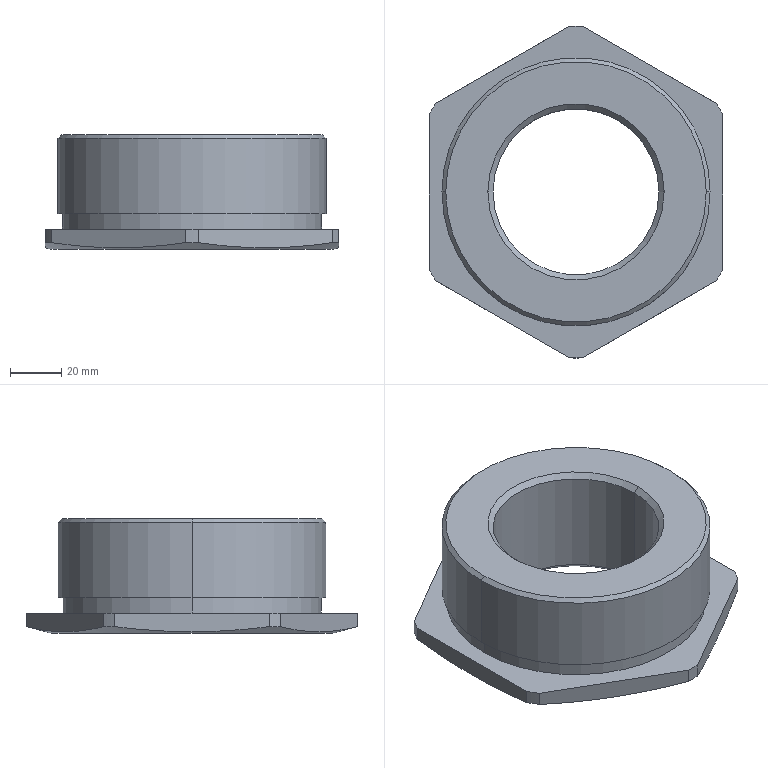Part | SolidWorks | features ICE 4, Chamfer 2, Extrusion 1 | 1 solid | 30 faces | box 115 x 130 x 45 mm | volume 256191 mm3 | cylinder 12 | plane 10 | cone 8 | commonest cylinder face diameters 130 x6 65 x2 101.5 x2 105 x2
STEP:
#1=CARTESIAN_POINT('',(55.,0.,0.));
#2=VERTEX_POINT('',#1);
#3=CARTESIAN_POINT('',(-55.,0.,0.));
#4=VERTEX_POINT('',#3);
#5=CARTESIAN_POINT('',(0.,0.,0.));
#6=DIRECTION('',(0.,0.,-1.));
#7=DIRECTION('',(-1.,0.,0.));
#8=AXIS2_PLACEMENT_3D('',#5,#6,#7);
#9=CIRCLE('',#8,55.);
#10=EDGE_CURVE('',#2,#4,#9,.T.);
#11=ORIENTED_EDGE('',*,*,#10,.F.);
#12=CARTESIAN_POINT('',(57.5,0.,0.6699));
#13=VERTEX_POINT('',#12);
#14=CARTESIAN_POINT('',(55.,0.,0.));
#15=DIRECTION('',(0.9659,0.,0.2588));
#16=VECTOR('',#15,1000.);
#17=LINE('',#14,#16);
#18=EDGE_CURVE('',#2,#13,#17,.T.);
#19=ORIENTED_EDGE('',*,*,#18,.T.);
#20=CARTESIAN_POINT('',(57.5,-30.311,2.679));
#21=VERTEX_POINT('',#20);
#22=CARTESIAN_POINT('',(57.5,0.,0.6699));
#23=CARTESIAN_POINT('',(57.5,-5.026,0.6699));
#24=CARTESIAN_POINT('',(57.5,-10.072,0.8493));
#25=CARTESIAN_POINT('',(57.5,-17.671,1.368));
#26=CARTESIAN_POINT('',(57.5,-20.211,1.582));
#27=CARTESIAN_POINT('',(57.5,-25.27,2.08));
#28=CARTESIAN_POINT('',(57.5,-27.793,2.365));
#29=CARTESIAN_POINT('',(57.5,-30.311,2.679));
#30=B_SPLINE_CURVE_WITH_KNOTS('',3,(#22,#23,#24,#25,#26,#27,#28,#29),.UNSPECIFIED.,.F.,.F.,(4,2,2,4),(0.09241,0.1074,0.1149,0.1224),.UNSPECIFIED.);
#31=EDGE_CURVE('',#13,#21,#30,.T.);
#32=ORIENTED_EDGE('',*,*,#31,.T.);
#33=CARTESIAN_POINT('',(55.,-34.641,2.679));
#34=VERTEX_POINT('',#33);
#35=CARTESIAN_POINT('',(0.,0.,2.679));
#36=DIRECTION('',(0.,0.,-1.));
#37=DIRECTION('',(1.,0.,0.));
#38=AXIS2_PLACEMENT_3D('',#35,#36,#37);
#39=CIRCLE('',#38,65.);
#40=EDGE_CURVE('',#21,#34,#39,.T.);
#41=ORIENTED_EDGE('',*,*,#40,.T.);
#42=CARTESIAN_POINT('',(2.5,-64.952,2.679));
#43=VERTEX_POINT('',#42);
#44=CARTESIAN_POINT('',(55.,-34.641,2.679));
#45=CARTESIAN_POINT('',(50.625,-37.167,2.048));
#46=CARTESIAN_POINT('',(46.25,-39.693,1.541));
#47=CARTESIAN_POINT('',(37.5,-44.745,0.8511));
#48=CARTESIAN_POINT('',(28.75,-49.796,0.4887));
#49=CARTESIAN_POINT('',(20.,-54.848,0.8511));
#50=CARTESIAN_POINT('',(11.25,-59.9,1.541));
#51=CARTESIAN_POINT('',(6.875,-62.426,2.048));
#52=CARTESIAN_POINT('',(2.5,-64.952,2.679));
#53=B_SPLINE_CURVE_WITH_KNOTS('',3,(#44,#45,#46,#47,#48,#49,#50,#51,#52),.UNSPECIFIED.,.F.,.F.,(4,2,1,2,4),(0.000000231,0.01516,0.03031,0.04547,0.06062),.UNSPECIFIED.);
#54=EDGE_CURVE('',#34,#43,#53,.T.);
#55=ORIENTED_EDGE('',*,*,#54,.T.);
#56=CARTESIAN_POINT('',(-2.5,-64.952,2.679));
#57=VERTEX_POINT('',#56);
#58=CARTESIAN_POINT('',(0.,0.,2.679));
#59=DIRECTION('',(0.,0.,-1.));
#60=DIRECTION('',(1.,0.,0.));
#61=AXIS2_PLACEMENT_3D('',#58,#59,#60);
#62=CIRCLE('',#61,65.);
#63=EDGE_CURVE('',#43,#57,#62,.T.);
#64=ORIENTED_EDGE('',*,*,#63,.T.);
#65=CARTESIAN_POINT('',(-55.,-34.641,2.679));
#66=VERTEX_POINT('',#65);
#67=CARTESIAN_POINT('',(-2.5,-64.952,2.679));
#68=CARTESIAN_POINT('',(-6.875,-62.426,2.048));
#69=CARTESIAN_POINT('',(-11.25,-59.9,1.541));
#70=CARTESIAN_POINT('',(-20.,-54.848,0.8511));
#71=CARTESIAN_POINT('',(-28.75,-49.796,0.4887));
#72=CARTESIAN_POINT('',(-37.5,-44.745,0.8511));
#73=CARTESIAN_POINT('',(-46.25,-39.693,1.541));
#74=CARTESIAN_POINT('',(-50.625,-37.167,2.048));
#75=CARTESIAN_POINT('',(-55.,-34.641,2.679));
#76=B_SPLINE_CURVE_WITH_KNOTS('',3,(#67,#68,#69,#70,#71,#72,#73,#74,#75),.UNSPECIFIED.,.F.,.F.,(4,2,1,2,4),(0.000000231,0.01516,0.03031,0.04547,0.06062),.UNSPECIFIED.);
#77=EDGE_CURVE('',#57,#66,#76,.T.);
#78=ORIENTED_EDGE('',*,*,#77,.T.);
#79=CARTESIAN_POINT('',(-57.5,-30.311,2.679));
#80=VERTEX_POINT('',#79);
#81=CARTESIAN_POINT('',(0.,0.,2.679));
#82=DIRECTION('',(0.,0.,-1.));
#83=DIRECTION('',(1.,0.,0.));
#84=AXIS2_PLACEMENT_3D('',#81,#82,#83);
#85=CIRCLE('',#84,65.);
#86=EDGE_CURVE('',#66,#80,#85,.T.);
#87=ORIENTED_EDGE('',*,*,#86,.T.);
#88=CARTESIAN_POINT('',(-57.5,0.,0.6699));
#89=VERTEX_POINT('',#88);
#90=CARTESIAN_POINT('',(-57.5,-30.311,2.679));
#91=CARTESIAN_POINT('',(-57.5,-25.293,2.053));
#92=CARTESIAN_POINT('',(-57.5,-20.261,1.546));
#93=CARTESIAN_POINT('',(-57.5,-10.16,0.8538));
#94=CARTESIAN_POINT('',(-57.5,-5.091,0.6699));
#95=CARTESIAN_POINT('',(-57.5,0.,0.6699));
#96=B_SPLINE_CURVE_WITH_KNOTS('',3,(#90,#91,#92,#93,#94,#95),.UNSPECIFIED.,.F.,.F.,(4,2,4),(0.06207,0.07724,0.09241),.UNSPECIFIED.);
#97=EDGE_CURVE('',#80,#89,#96,.T.);
#98=ORIENTED_EDGE('',*,*,#97,.T.);
#99=CARTESIAN_POINT('',(-55.,0.,0.));
#100=DIRECTION('',(-0.9659,0.,0.2588));
#101=VECTOR('',#100,1000.);
#102=LINE('',#99,#101);
#103=EDGE_CURVE('',#4,#89,#102,.T.);
#104=ORIENTED_EDGE('',*,*,#103,.F.);
#105=EDGE_LOOP('',(#11,#19,#32,#41,#55,#64,#78,#87,#98,#104));
#106=FACE_OUTER_BOUND('',#105,.T.);
#107=CARTESIAN_POINT('',(0.,0.,0.));
#108=DIRECTION('',(0.,0.,1.));
#109=DIRECTION('',(-1.,0.,0.));
#110=AXIS2_PLACEMENT_3D('',#107,#108,#109);
#111=CONICAL_SURFACE('',#110,55.,1.309);
#112=ADVANCED_FACE('',(#106),#111,.T.);
#113=CARTESIAN_POINT('',(51.,0.,45.));
#114=VERTEX_POINT('',#113);
#115=CARTESIAN_POINT('',(-51.,0.,45.));
#116=VERTEX_POINT('',#115);
#117=CARTESIAN_POINT('',(0.,0.,45.));
#118=DIRECTION('',(0.,0.,1.));
#119=DIRECTION('',(-1.,0.,0.));
#120=AXIS2_PLACEMENT_3D('',#117,#118,#119);
#121=CIRCLE('',#120,51.);
#122=EDGE_CURVE('',#114,#116,#121,.T.);
#123=ORIENTED_EDGE('',*,*,#122,.F.);
#124=CARTESIAN_POINT('',(52.5,0.,43.5));
#125=VERTEX_POINT('',#124);
#126=CARTESIAN_POINT('',(52.5,0.,43.5));
#127=DIRECTION('',(0.7071,0.,-0.7071));
#128=VECTOR('',#127,1000.);
#129=LINE('',#126,#128);
#130=EDGE_CURVE('',#114,#125,#129,.T.);
#131=ORIENTED_EDGE('',*,*,#130,.T.);
#132=CARTESIAN_POINT('',(-52.5,0.,43.5));
#133=VERTEX_POINT('',#132);
#134=CARTESIAN_POINT('',(0.,0.,43.5));
#135=DIRECTION('',(0.,0.,-1.));
#136=DIRECTION('',(-1.,0.,0.));
#137=AXIS2_PLACEMENT_3D('',#134,#135,#136);
#138=CIRCLE('',#137,52.5);
#139=EDGE_CURVE('',#133,#125,#138,.T.);
#140=ORIENTED_EDGE('',*,*,#139,.F.);
#141=CARTESIAN_POINT('',(-52.5,0.,43.5));
#142=DIRECTION('',(-0.7071,0.,-0.7071));
#143=VECTOR('',#142,1000.);
#144=LINE('',#141,#143);
#145=EDGE_CURVE('',#116,#133,#144,.T.);
#146=ORIENTED_EDGE('',*,*,#145,.F.);
#147=EDGE_LOOP('',(#123,#131,#140,#146));
#148=FACE_OUTER_BOUND('',#147,.T.);
#149=CARTESIAN_POINT('',(0.,0.,43.5));
#150=DIRECTION('',(0.,0.,-1.));
#151=DIRECTION('',(-1.,0.,0.));
#152=AXIS2_PLACEMENT_3D('',#149,#150,#151);
#153=CONICAL_SURFACE('',#152,52.5,0.7854);
#154=ADVANCED_FACE('',(#148),#153,.T.);
#155=CARTESIAN_POINT('',(32.5,0.,2.));
#156=VERTEX_POINT('',#155);
#157=CARTESIAN_POINT('',(-32.5,0.,2.));
#158=VERTEX_POINT('',#157);
#159=CARTESIAN_POINT('',(0.,0.,2.));
#160=DIRECTION('',(0.,0.,-1.));
#161=DIRECTION('',(1.,0.,0.));
#162=AXIS2_PLACEMENT_3D('',#159,#160,#161);
#163=CIRCLE('',#162,32.5);
#164=EDGE_CURVE('',#156,#158,#163,.T.);
#165=ORIENTED_EDGE('',*,*,#164,.F.);
#166=CARTESIAN_POINT('',(34.5,0.,0.));
#167=VERTEX_POINT('',#166);
#168=CARTESIAN_POINT('',(34.5,0.,0.));
#169=DIRECTION('',(0.7071,0.,-0.7071));
#170=VECTOR('',#169,1000.);
#171=LINE('',#168,#170);
#172=EDGE_CURVE('',#156,#167,#171,.T.);
#173=ORIENTED_EDGE('',*,*,#172,.T.);
#174=CARTESIAN_POINT('',(-34.5,0.,0.));
#175=VERTEX_POINT('',#174);
#176=CARTESIAN_POINT('',(0.,0.,0.));
#177=DIRECTION('',(0.,0.,1.));
#178=DIRECTION('',(1.,0.,0.));
#179=AXIS2_PLACEMENT_3D('',#176,#177,#178);
#180=CIRCLE('',#179,34.5);
#181=EDGE_CURVE('',#175,#167,#180,.T.);
#182=ORIENTED_EDGE('',*,*,#181,.F.);
#183=CARTESIAN_POINT('',(-34.5,0.,0.));
#184=DIRECTION('',(-0.7071,0.,-0.7071));
#185=VECTOR('',#184,1000.);
#186=LINE('',#183,#185);
#187=EDGE_CURVE('',#158,#175,#186,.T.);
#188=ORIENTED_EDGE('',*,*,#187,.F.);
#189=EDGE_LOOP('',(#165,#173,#182,#188));
#190=FACE_OUTER_BOUND('',#189,.T.);
#191=CARTESIAN_POINT('',(0.,0.,0.));
#192=DIRECTION('',(0.,0.,-1.));
#193=DIRECTION('',(-1.,0.,0.));
#194=AXIS2_PLACEMENT_3D('',#191,#192,#193);
#195=CONICAL_SURFACE('',#194,34.5,0.7854);
#196=ADVANCED_FACE('',(#190),#195,.F.);
#197=CARTESIAN_POINT('',(-32.5,0.,43.));
#198=VERTEX_POINT('',#197);
#199=CARTESIAN_POINT('',(32.5,0.,43.));
#200=VERTEX_POINT('',#199);
#201=CARTESIAN_POINT('',(0.,0.,43.));
#202=DIRECTION('',(0.,0.,1.));
#203=DIRECTION('',(-1.,0.,0.));
#204=AXIS2_PLACEMENT_3D('',#201,#202,#203);
#205=CIRCLE('',#204,32.5);
#206=EDGE_CURVE('',#198,#200,#205,.T.);
#207=ORIENTED_EDGE('',*,*,#206,.F.);
#208=CARTESIAN_POINT('',(-34.5,0.,45.));
#209=VERTEX_POINT('',#208);
#210=CARTESIAN_POINT('',(-32.5,0.,43.));
#211=DIRECTION('',(-0.7071,0.,0.7071));
#212=VECTOR('',#211,1000.);
#213=LINE('',#210,#212);
#214=EDGE_CURVE('',#198,#209,#213,.T.);
#215=ORIENTED_EDGE('',*,*,#214,.T.);
#216=CARTESIAN_POINT('',(34.5,0.,45.));
#217=VERTEX_POINT('',#216);
#218=CARTESIAN_POINT('',(0.,0.,45.));
#219=DIRECTION('',(0.,0.,-1.));
#220=DIRECTION('',(-1.,0.,0.));
#221=AXIS2_PLACEMENT_3D('',#218,#219,#220);
#222=CIRCLE('',#221,34.5);
#223=EDGE_CURVE('',#217,#209,#222,.T.);
#224=ORIENTED_EDGE('',*,*,#223,.F.);
#225=CARTESIAN_POINT('',(32.5,0.,43.));
#226=DIRECTION('',(0.7071,0.,0.7071));
#227=VECTOR('',#226,1000.);
#228=LINE('',#225,#227);
#229=EDGE_CURVE('',#200,#217,#228,.T.);
#230=ORIENTED_EDGE('',*,*,#229,.F.);
#231=EDGE_LOOP('',(#207,#215,#224,#230));
#232=FACE_OUTER_BOUND('',#231,.T.);
#233=CARTESIAN_POINT('',(0.,0.,43.));
#234=DIRECTION('',(0.,0.,1.));
#235=DIRECTION('',(1.,0.,0.));
#236=AXIS2_PLACEMENT_3D('',#233,#234,#235);
#237=CONICAL_SURFACE('',#236,32.5,0.7854);
#238=ADVANCED_FACE('',(#232),#237,.F.);
#239=ORIENTED_EDGE('',*,*,#164,.T.);
#240=CARTESIAN_POINT('',(-32.5,0.,0.));
#241=DIRECTION('',(0.,0.,1.));
#242=VECTOR('',#241,1000.);
#243=LINE('',#240,#242);
#244=EDGE_CURVE('',#158,#198,#243,.T.);
#245=ORIENTED_EDGE('',*,*,#244,.T.);
#246=ORIENTED_EDGE('',*,*,#206,.T.);
#247=CARTESIAN_POINT('',(32.5,0.,0.));
#248=DIRECTION('',(0.,0.,1.));
#249=VECTOR('',#248,1000.);
#250=LINE('',#247,#249);
#251=EDGE_CURVE('',#156,#200,#250,.T.);
#252=ORIENTED_EDGE('',*,*,#251,.F.);
#253=EDGE_LOOP('',(#239,#245,#246,#252));
#254=FACE_OUTER_BOUND('',#253,.T.);
#255=CARTESIAN_POINT('',(0.,0.,0.));
#256=DIRECTION('',(0.,0.,1.));
#257=DIRECTION('',(1.,0.,0.));
#258=AXIS2_PLACEMENT_3D('',#255,#256,#257);
#259=CYLINDRICAL_SURFACE('',#258,32.5);
#260=ADVANCED_FACE('',(#254),#259,.F.);
#261=ORIENTED_EDGE('',*,*,#139,.T.);
#262=CARTESIAN_POINT('',(52.5,0.,14.));
#263=VERTEX_POINT('',#262);
#264=CARTESIAN_POINT('',(52.5,0.,45.));
#265=DIRECTION('',(0.,0.,-1.));
#266=VECTOR('',#265,1000.);
#267=LINE('',#264,#266);
#268=EDGE_CURVE('',#125,#263,#267,.T.);
#269=ORIENTED_EDGE('',*,*,#268,.T.);
#270=CARTESIAN_POINT('',(-52.5,0.,14.));
#271=VERTEX_POINT('',#270);
#272=CARTESIAN_POINT('',(0.,0.,14.));
#273=DIRECTION('',(0.,0.,1.));
#274=DIRECTION('',(1.,0.,0.));
#275=AXIS2_PLACEMENT_3D('',#272,#273,#274);
#276=CIRCLE('',#275,52.5);
#277=EDGE_CURVE('',#263,#271,#276,.T.);
#278=ORIENTED_EDGE('',*,*,#277,.T.);
#279=CARTESIAN_POINT('',(-52.5,0.,45.));
#280=DIRECTION('',(0.,0.,-1.));
#281=VECTOR('',#280,1000.);
#282=LINE('',#279,#281);
#283=EDGE_CURVE('',#133,#271,#282,.T.);
#284=ORIENTED_EDGE('',*,*,#283,.F.);
#285=EDGE_LOOP('',(#261,#269,#278,#284));
#286=FACE_OUTER_BOUND('',#285,.T.);
#287=CARTESIAN_POINT('',(0.,0.,45.));
#288=DIRECTION('',(0.,0.,-1.));
#289=DIRECTION('',(-1.,0.,0.));
#290=AXIS2_PLACEMENT_3D('',#287,#288,#289);
#291=CYLINDRICAL_SURFACE('',#290,52.5);
#292=ADVANCED_FACE('',(#286),#291,.T.);
#293=CARTESIAN_POINT('',(50.75,0.,14.));
#294=VERTEX_POINT('',#293);
#295=CARTESIAN_POINT('',(-50.75,0.,14.));
#296=VERTEX_POINT('',#295);
#297=CARTESIAN_POINT('',(0.,0.,14.));
#298=DIRECTION('',(0.,0.,1.));
#299=DIRECTION('',(1.,0.,0.));
#300=AXIS2_PLACEMENT_3D('',#297,#298,#299);
#301=CIRCLE('',#300,50.75);
#302=EDGE_CURVE('',#294,#296,#301,.T.);
#303=ORIENTED_EDGE('',*,*,#302,.F.);
#304=CARTESIAN_POINT('',(50.75,0.,8.));
#305=VERTEX_POINT('',#304);
#306=CARTESIAN_POINT('',(50.75,0.,14.));
#307=DIRECTION('',(0.,0.,-1.));
#308=VECTOR('',#307,1000.);
#309=LINE('',#306,#308);
#310=EDGE_CURVE('',#294,#305,#309,.T.);
#311=ORIENTED_EDGE('',*,*,#310,.T.);
#312=CARTESIAN_POINT('',(-50.75,0.,8.));
#313=VERTEX_POINT('',#312);
#314=CARTESIAN_POINT('',(0.,0.,8.));
#315=DIRECTION('',(0.,0.,1.));
#316=DIRECTION('',(1.,0.,0.));
#317=AXIS2_PLACEMENT_3D('',#314,#315,#316);
#318=CIRCLE('',#317,50.75);
#319=EDGE_CURVE('',#305,#313,#318,.T.);
#320=ORIENTED_EDGE('',*,*,#319,.T.);
#321=CARTESIAN_POINT('',(-50.75,0.,14.));
#322=DIRECTION('',(0.,0.,-1.));
#323=VECTOR('',#322,1000.);
#324=LINE('',#321,#323);
#325=EDGE_CURVE('',#296,#313,#324,.T.);
#326=ORIENTED_EDGE('',*,*,#325,.F.);
#327=EDGE_LOOP('',(#303,#311,#320,#326));
#328=FACE_OUTER_BOUND('',#327,.T.);
#329=CARTESIAN_POINT('',(0.,0.,14.));
#330=DIRECTION('',(0.,0.,-1.));
#331=DIRECTION('',(-1.,0.,0.));
#332=AXIS2_PLACEMENT_3D('',#329,#330,#331);
#333=CYLINDRICAL_SURFACE('',#332,50.75);
#334=ADVANCED_FACE('',(#328),#333,.T.);
#335=CARTESIAN_POINT('',(57.5,30.311,2.679));
#336=VERTEX_POINT('',#335);
#337=CARTESIAN_POINT('',(57.5,30.311,2.679));
#338=CARTESIAN_POINT('',(57.5,25.293,2.053));
#339=CARTESIAN_POINT('',(57.5,20.261,1.546));
#340=CARTESIAN_POINT('',(57.5,10.16,0.8538));
#341=CARTESIAN_POINT('',(57.5,5.091,0.6699));
#342=CARTESIAN_POINT('',(57.5,0.,0.6699));
#343=B_SPLINE_CURVE_WITH_KNOTS('',3,(#337,#338,#339,#340,#341,#342),.UNSPECIFIED.,.F.,.F.,(4,2,4),(0.06207,0.07724,0.09241),.UNSPECIFIED.);
#344=EDGE_CURVE('',#336,#13,#343,.T.);
#345=ORIENTED_EDGE('',*,*,#344,.F.);
#346=CARTESIAN_POINT('',(57.5,30.311,8.));
#347=VERTEX_POINT('',#346);
#348=CARTESIAN_POINT('',(57.5,30.311,8.));
#349=DIRECTION('',(0.,0.,-1.));
#350=VECTOR('',#349,1000.);
#351=LINE('',#348,#350);
#352=EDGE_CURVE('',#347,#336,#351,.T.);
#353=ORIENTED_EDGE('',*,*,#352,.F.);
#354=CARTESIAN_POINT('',(57.5,-30.311,8.));
#355=VERTEX_POINT('',#354);
#356=CARTESIAN_POINT('',(57.5,0.,8.));
#357=DIRECTION('',(0.,1.,0.));
#358=VECTOR('',#357,1000.);
#359=LINE('',#356,#358);
#360=EDGE_CURVE('',#355,#347,#359,.T.);
#361=ORIENTED_EDGE('',*,*,#360,.F.);
#362=CARTESIAN_POINT('',(57.5,-30.311,8.));
#363=DIRECTION('',(0.,0.,-1.));
#364=VECTOR('',#363,1000.);
#365=LINE('',#362,#364);
#366=EDGE_CURVE('',#355,#21,#365,.T.);
#367=ORIENTED_EDGE('',*,*,#366,.T.);
#368=ORIENTED_EDGE('',*,*,#31,.F.);
#369=EDGE_LOOP('',(#345,#353,#361,#367,#368));
#370=FACE_OUTER_BOUND('',#369,.T.);
#371=CARTESIAN_POINT('',(57.5,0.,8.));
#372=DIRECTION('',(-1.,0.,0.));
#373=DIRECTION('',(0.,-1.,0.));
#374=AXIS2_PLACEMENT_3D('',#371,#372,#373);
#375=PLANE('',#374);
#376=ADVANCED_FACE('',(#370),#375,.F.);
#377=CARTESIAN_POINT('',(55.,34.641,2.679));
#378=VERTEX_POINT('',#377);
#379=CARTESIAN_POINT('',(0.,0.,2.679));
#380=DIRECTION('',(0.,0.,-1.));
#381=DIRECTION('',(1.,0.,0.));
#382=AXIS2_PLACEMENT_3D('',#379,#380,#381);
#383=CIRCLE('',#382,65.);
#384=EDGE_CURVE('',#378,#336,#383,.T.);
#385=ORIENTED_EDGE('',*,*,#384,.F.);
#386=CARTESIAN_POINT('',(55.,34.641,8.));
#387=VERTEX_POINT('',#386);
#388=CARTESIAN_POINT('',(55.,34.641,8.));
#389=DIRECTION('',(0.,0.,-1.));
#390=VECTOR('',#389,1000.);
#391=LINE('',#388,#390);
#392=EDGE_CURVE('',#387,#378,#391,.T.);
#393=ORIENTED_EDGE('',*,*,#392,.F.);
#394=CARTESIAN_POINT('',(0.,0.,8.));
#395=DIRECTION('',(0.,0.,1.));
#396=DIRECTION('',(1.,0.,0.));
#397=AXIS2_PLACEMENT_3D('',#394,#395,#396);
#398=CIRCLE('',#397,65.);
#399=EDGE_CURVE('',#347,#387,#398,.T.);
#400=ORIENTED_EDGE('',*,*,#399,.F.);
#401=ORIENTED_EDGE('',*,*,#352,.T.);
#402=EDGE_LOOP('',(#385,#393,#400,#401));
#403=FACE_OUTER_BOUND('',#402,.T.);
#404=CARTESIAN_POINT('',(0.,0.,8.));
#405=DIRECTION('',(0.,0.,-1.));
#406=DIRECTION('',(-1.,0.,0.));
#407=AXIS2_PLACEMENT_3D('',#404,#405,#406);
#408=CYLINDRICAL_SURFACE('',#407,65.);
#409=ADVANCED_FACE('',(#403),#408,.T.);
#410=CARTESIAN_POINT('',(2.5,64.952,2.679));
#411=VERTEX_POINT('',#410);
#412=CARTESIAN_POINT('',(2.5,64.952,2.679));
#413=CARTESIAN_POINT('',(6.875,62.426,2.048));
#414=CARTESIAN_POINT('',(11.25,59.9,1.541));
#415=CARTESIAN_POINT('',(20.,54.848,0.8511));
#416=CARTESIAN_POINT('',(28.75,49.796,0.4887));
#417=CARTESIAN_POINT('',(37.5,44.745,0.8511));
#418=CARTESIAN_POINT('',(46.25,39.693,1.541));
#419=CARTESIAN_POINT('',(50.625,37.167,2.048));
#420=CARTESIAN_POINT('',(55.,34.641,2.679));
#421=B_SPLINE_CURVE_WITH_KNOTS('',3,(#412,#413,#414,#415,#416,#417,#418,#419,#420),.UNSPECIFIED.,.F.,.F.,(4,2,1,2,4),(0.000000231,0.01516,0.03031,0.04547,0.06062),.UNSPECIFIED.);
#422=EDGE_CURVE('',#411,#378,#421,.T.);
#423=ORIENTED_EDGE('',*,*,#422,.F.);
#424=CARTESIAN_POINT('',(2.5,64.952,8.));
#425=VERTEX_POINT('',#424);
#426=CARTESIAN_POINT('',(2.5,64.952,8.));
#427=DIRECTION('',(0.,0.,-1.));
#428=VECTOR('',#427,1000.);
#429=LINE('',#426,#428);
#430=EDGE_CURVE('',#425,#411,#429,.T.);
#431=ORIENTED_EDGE('',*,*,#430,.F.);
#432=CARTESIAN_POINT('',(28.75,49.796,8.));
#433=DIRECTION('',(-0.866,0.5,0.));
#434=VECTOR('',#433,1000.);
#435=LINE('',#432,#434);
#436=EDGE_CURVE('',#387,#425,#435,.T.);
#437=ORIENTED_EDGE('',*,*,#436,.F.);
#438=ORIENTED_EDGE('',*,*,#392,.T.);
#439=EDGE_LOOP('',(#423,#431,#437,#438));
#440=FACE_OUTER_BOUND('',#439,.T.);
#441=CARTESIAN_POINT('',(28.75,49.796,8.));
#442=DIRECTION('',(-0.5,-0.866,0.));
#443=DIRECTION('',(0.866,-0.5,0.));
#444=AXIS2_PLACEMENT_3D('',#441,#442,#443);
#445=PLANE('',#444);
#446=ADVANCED_FACE('',(#440),#445,.F.);
#447=CARTESIAN_POINT('',(-2.5,64.952,2.679));
#448=VERTEX_POINT('',#447);
#449=CARTESIAN_POINT('',(0.,0.,2.679));
#450=DIRECTION('',(0.,0.,-1.));
#451=DIRECTION('',(1.,0.,0.));
#452=AXIS2_PLACEMENT_3D('',#449,#450,#451);
#453=CIRCLE('',#452,65.);
#454=EDGE_CURVE('',#448,#411,#453,.T.);
#455=ORIENTED_EDGE('',*,*,#454,.F.);
#456=CARTESIAN_POINT('',(-2.5,64.952,8.));
#457=VERTEX_POINT('',#456);
#458=CARTESIAN_POINT('',(-2.5,64.952,8.));
#459=DIRECTION('',(0.,0.,-1.));
#460=VECTOR('',#459,1000.);
#461=LINE('',#458,#460);
#462=EDGE_CURVE('',#457,#448,#461,.T.);
#463=ORIENTED_EDGE('',*,*,#462,.F.);
#464=CARTESIAN_POINT('',(0.,0.,8.));
#465=DIRECTION('',(0.,0.,1.));
#466=DIRECTION('',(1.,0.,0.));
#467=AXIS2_PLACEMENT_3D('',#464,#465,#466);
#468=CIRCLE('',#467,65.);
#469=EDGE_CURVE('',#425,#457,#468,.T.);
#470=ORIENTED_EDGE('',*,*,#469,.F.);
#471=ORIENTED_EDGE('',*,*,#430,.T.);
#472=EDGE_LOOP('',(#455,#463,#470,#471));
#473=FACE_OUTER_BOUND('',#472,.T.);
#474=CARTESIAN_POINT('',(0.,0.,8.));
#475=DIRECTION('',(0.,0.,-1.));
#476=DIRECTION('',(-1.,0.,0.));
#477=AXIS2_PLACEMENT_3D('',#474,#475,#476);
#478=CYLINDRICAL_SURFACE('',#477,65.);
#479=ADVANCED_FACE('',(#473),#478,.T.);
#480=CARTESIAN_POINT('',(-55.,34.641,2.679));
#481=VERTEX_POINT('',#480);
#482=CARTESIAN_POINT('',(-55.,34.641,2.679));
#483=CARTESIAN_POINT('',(-50.625,37.167,2.048));
#484=CARTESIAN_POINT('',(-46.25,39.693,1.541));
#485=CARTESIAN_POINT('',(-37.5,44.745,0.8511));
#486=CARTESIAN_POINT('',(-28.75,49.796,0.4887));
#487=CARTESIAN_POINT('',(-20.,54.848,0.8511));
#488=CARTESIAN_POINT('',(-11.25,59.9,1.541));
#489=CARTESIAN_POINT('',(-6.875,62.426,2.048));
#490=CARTESIAN_POINT('',(-2.5,64.952,2.679));
#491=B_SPLINE_CURVE_WITH_KNOTS('',3,(#482,#483,#484,#485,#486,#487,#488,#489,#490),.UNSPECIFIED.,.F.,.F.,(4,2,1,2,4),(0.000000231,0.01516,0.03031,0.04547,0.06062),.UNSPECIFIED.);
#492=EDGE_CURVE('',#481,#448,#491,.T.);
#493=ORIENTED_EDGE('',*,*,#492,.F.);
#494=CARTESIAN_POINT('',(-55.,34.641,8.));
#495=VERTEX_POINT('',#494);
#496=CARTESIAN_POINT('',(-55.,34.641,8.));
#497=DIRECTION('',(0.,0.,-1.));
#498=VECTOR('',#497,1000.);
#499=LINE('',#496,#498);
#500=EDGE_CURVE('',#495,#481,#499,.T.);
#501=ORIENTED_EDGE('',*,*,#500,.F.);
#502=CARTESIAN_POINT('',(-28.75,49.796,8.));
#503=DIRECTION('',(-0.866,-0.5,0.));
#504=VECTOR('',#503,1000.);
#505=LINE('',#502,#504);
#506=EDGE_CURVE('',#457,#495,#505,.T.);
#507=ORIENTED_EDGE('',*,*,#506,.F.);
#508=ORIENTED_EDGE('',*,*,#462,.T.);
#509=EDGE_LOOP('',(#493,#501,#507,#508));
#510=FACE_OUTER_BOUND('',#509,.T.);
#511=CARTESIAN_POINT('',(-28.75,49.796,8.));
#512=DIRECTION('',(0.5,-0.866,0.));
#513=DIRECTION('',(0.866,0.5,0.));
#514=AXIS2_PLACEMENT_3D('',#511,#512,#513);
#515=PLANE('',#514);
#516=ADVANCED_FACE('',(#510),#515,.F.);
#517=CARTESIAN_POINT('',(-57.5,30.311,2.679));
#518=VERTEX_POINT('',#517);
#519=CARTESIAN_POINT('',(0.,0.,2.679));
#520=DIRECTION('',(0.,0.,-1.));
#521=DIRECTION('',(1.,0.,0.));
#522=AXIS2_PLACEMENT_3D('',#519,#520,#521);
#523=CIRCLE('',#522,65.);
#524=EDGE_CURVE('',#518,#481,#523,.T.);
#525=ORIENTED_EDGE('',*,*,#524,.F.);
#526=CARTESIAN_POINT('',(-57.5,30.311,8.));
#527=VERTEX_POINT('',#526);
#528=CARTESIAN_POINT('',(-57.5,30.311,8.));
#529=DIRECTION('',(0.,0.,-1.));
#530=VECTOR('',#529,1000.);
#531=LINE('',#528,#530);
#532=EDGE_CURVE('',#527,#518,#531,.T.);
#533=ORIENTED_EDGE('',*,*,#532,.F.);
#534=CARTESIAN_POINT('',(0.,0.,8.));
#535=DIRECTION('',(0.,0.,1.));
#536=DIRECTION('',(1.,0.,0.));
#537=AXIS2_PLACEMENT_3D('',#534,#535,#536);
#538=CIRCLE('',#537,65.);
#539=EDGE_CURVE('',#495,#527,#538,.T.);
#540=ORIENTED_EDGE('',*,*,#539,.F.);
#541=ORIENTED_EDGE('',*,*,#500,.T.);
#542=EDGE_LOOP('',(#525,#533,#540,#541));
#543=FACE_OUTER_BOUND('',#542,.T.);
#544=CARTESIAN_POINT('',(0.,0.,8.));
#545=DIRECTION('',(0.,0.,-1.));
#546=DIRECTION('',(-1.,0.,0.));
#547=AXIS2_PLACEMENT_3D('',#544,#545,#546);
#548=CYLINDRICAL_SURFACE('',#547,65.);
#549=ADVANCED_FACE('',(#543),#548,.T.);
#550=ORIENTED_EDGE('',*,*,#97,.F.);
#551=CARTESIAN_POINT('',(-57.5,-30.311,8.));
#552=VERTEX_POINT('',#551);
#553=CARTESIAN_POINT('',(-57.5,-30.311,8.));
#554=DIRECTION('',(0.,0.,-1.));
#555=VECTOR('',#554,1000.);
#556=LINE('',#553,#555);
#557=EDGE_CURVE('',#552,#80,#556,.T.);
#558=ORIENTED_EDGE('',*,*,#557,.F.);
#559=CARTESIAN_POINT('',(-57.5,0.,8.));
#560=DIRECTION('',(0.,-1.,0.));
#561=VECTOR('',#560,1000.);
#562=LINE('',#559,#561);
#563=EDGE_CURVE('',#527,#552,#562,.T.);
#564=ORIENTED_EDGE('',*,*,#563,.F.);
#565=ORIENTED_EDGE('',*,*,#532,.T.);
#566=CARTESIAN_POINT('',(-57.5,0.,0.6699));
#567=CARTESIAN_POINT('',(-57.5,5.026,0.6699));
#568=CARTESIAN_POINT('',(-57.5,10.072,0.8493));
#569=CARTESIAN_POINT('',(-57.5,17.671,1.368));
#570=CARTESIAN_POINT('',(-57.5,20.211,1.582));
#571=CARTESIAN_POINT('',(-57.5,25.27,2.08));
#572=CARTESIAN_POINT('',(-57.5,27.793,2.365));
#573=CARTESIAN_POINT('',(-57.5,30.311,2.679));
#574=B_SPLINE_CURVE_WITH_KNOTS('',3,(#566,#567,#568,#569,#570,#571,#572,#573),.UNSPECIFIED.,.F.,.F.,(4,2,2,4),(0.09241,0.1074,0.1149,0.1224),.UNSPECIFIED.);
#575=EDGE_CURVE('',#89,#518,#574,.T.);
#576=ORIENTED_EDGE('',*,*,#575,.F.);
#577=EDGE_LOOP('',(#550,#558,#564,#565,#576));
#578=FACE_OUTER_BOUND('',#577,.T.);
#579=CARTESIAN_POINT('',(-57.5,0.,8.));
#580=DIRECTION('',(1.,0.,0.));
#581=DIRECTION('',(0.,0.,-1.));
#582=AXIS2_PLACEMENT_3D('',#579,#580,#581);
#583=PLANE('',#582);
#584=ADVANCED_FACE('',(#578),#583,.F.);
#585=ORIENTED_EDGE('',*,*,#86,.F.);
#586=CARTESIAN_POINT('',(-55.,-34.641,8.));
#587=VERTEX_POINT('',#586);
#588=CARTESIAN_POINT('',(-55.,-34.641,8.));
#589=DIRECTION('',(0.,0.,-1.));
#590=VECTOR('',#589,1000.);
#591=LINE('',#588,#590);
#592=EDGE_CURVE('',#587,#66,#591,.T.);
#593=ORIENTED_EDGE('',*,*,#592,.F.);
#594=CARTESIAN_POINT('',(0.,0.,8.));
#595=DIRECTION('',(0.,0.,1.));
#596=DIRECTION('',(1.,0.,0.));
#597=AXIS2_PLACEMENT_3D('',#594,#595,#596);
#598=CIRCLE('',#597,65.);
#599=EDGE_CURVE('',#552,#587,#598,.T.);
#600=ORIENTED_EDGE('',*,*,#599,.F.);
#601=ORIENTED_EDGE('',*,*,#557,.T.);
#602=EDGE_LOOP('',(#585,#593,#600,#601));
#603=FACE_OUTER_BOUND('',#602,.T.);
#604=CARTESIAN_POINT('',(0.,0.,8.));
#605=DIRECTION('',(0.,0.,-1.));
#606=DIRECTION('',(-1.,0.,0.));
#607=AXIS2_PLACEMENT_3D('',#604,#605,#606);
#608=CYLINDRICAL_SURFACE('',#607,65.);
#609=ADVANCED_FACE('',(#603),#608,.T.);
#610=ORIENTED_EDGE('',*,*,#77,.F.);
#611=CARTESIAN_POINT('',(-2.5,-64.952,8.));
#612=VERTEX_POINT('',#611);
#613=CARTESIAN_POINT('',(-2.5,-64.952,8.));
#614=DIRECTION('',(0.,0.,-1.));
#615=VECTOR('',#614,1000.);
#616=LINE('',#613,#615);
#617=EDGE_CURVE('',#612,#57,#616,.T.);
#618=ORIENTED_EDGE('',*,*,#617,.F.);
#619=CARTESIAN_POINT('',(-28.75,-49.796,8.));
#620=DIRECTION('',(0.866,-0.5,0.));
#621=VECTOR('',#620,1000.);
#622=LINE('',#619,#621);
#623=EDGE_CURVE('',#587,#612,#622,.T.);
#624=ORIENTED_EDGE('',*,*,#623,.F.);
#625=ORIENTED_EDGE('',*,*,#592,.T.);
#626=EDGE_LOOP('',(#610,#618,#624,#625));
#627=FACE_OUTER_BOUND('',#626,.T.);
#628=CARTESIAN_POINT('',(-28.75,-49.796,8.));
#629=DIRECTION('',(0.5,0.866,0.));
#630=DIRECTION('',(-0.866,0.5,0.));
#631=AXIS2_PLACEMENT_3D('',#628,#629,#630);
#632=PLANE('',#631);
#633=ADVANCED_FACE('',(#627),#632,.F.);
#634=ORIENTED_EDGE('',*,*,#63,.F.);
#635=CARTESIAN_POINT('',(2.5,-64.952,8.));
#636=VERTEX_POINT('',#635);
#637=CARTESIAN_POINT('',(2.5,-64.952,8.));
#638=DIRECTION('',(0.,0.,-1.));
#639=VECTOR('',#638,1000.);
#640=LINE('',#637,#639);
#641=EDGE_CURVE('',#636,#43,#640,.T.);
#642=ORIENTED_EDGE('',*,*,#641,.F.);
#643=CARTESIAN_POINT('',(0.,0.,8.));
#644=DIRECTION('',(0.,0.,1.));
#645=DIRECTION('',(1.,0.,0.));
#646=AXIS2_PLACEMENT_3D('',#643,#644,#645);
#647=CIRCLE('',#646,65.);
#648=EDGE_CURVE('',#612,#636,#647,.T.);
#649=ORIENTED_EDGE('',*,*,#648,.F.);
#650=ORIENTED_EDGE('',*,*,#617,.T.);
#651=EDGE_LOOP('',(#634,#642,#649,#650));
#652=FACE_OUTER_BOUND('',#651,.T.);
#653=CARTESIAN_POINT('',(0.,0.,8.));
#654=DIRECTION('',(0.,0.,-1.));
#655=DIRECTION('',(-1.,0.,0.));
#656=AXIS2_PLACEMENT_3D('',#653,#654,#655);
#657=CYLINDRICAL_SURFACE('',#656,65.);
#658=ADVANCED_FACE('',(#652),#657,.T.);
#659=ORIENTED_EDGE('',*,*,#54,.F.);
#660=CARTESIAN_POINT('',(55.,-34.641,8.));
#661=VERTEX_POINT('',#660);
#662=CARTESIAN_POINT('',(55.,-34.641,8.));
#663=DIRECTION('',(0.,0.,-1.));
#664=VECTOR('',#663,1000.);
#665=LINE('',#662,#664);
#666=EDGE_CURVE('',#661,#34,#665,.T.);
#667=ORIENTED_EDGE('',*,*,#666,.F.);
#668=CARTESIAN_POINT('',(28.75,-49.796,8.));
#669=DIRECTION('',(0.866,0.5,0.));
#670=VECTOR('',#669,1000.);
#671=LINE('',#668,#670);
#672=EDGE_CURVE('',#636,#661,#671,.T.);
#673=ORIENTED_EDGE('',*,*,#672,.F.);
#674=ORIENTED_EDGE('',*,*,#641,.T.);
#675=EDGE_LOOP('',(#659,#667,#673,#674));
#676=FACE_OUTER_BOUND('',#675,.T.);
#677=CARTESIAN_POINT('',(28.75,-49.796,8.));
#678=DIRECTION('',(-0.5,0.866,0.));
#679=DIRECTION('',(-0.866,-0.5,0.));
#680=AXIS2_PLACEMENT_3D('',#677,#678,#679);
#681=PLANE('',#680);
#682=ADVANCED_FACE('',(#676),#681,.F.);
#683=ORIENTED_EDGE('',*,*,#40,.F.);
#684=ORIENTED_EDGE('',*,*,#366,.F.);
#685=CARTESIAN_POINT('',(0.,0.,8.));
#686=DIRECTION('',(0.,0.,1.));
#687=DIRECTION('',(1.,0.,0.));
#688=AXIS2_PLACEMENT_3D('',#685,#686,#687);
#689=CIRCLE('',#688,65.);
#690=EDGE_CURVE('',#661,#355,#689,.T.);
#691=ORIENTED_EDGE('',*,*,#690,.F.);
#692=ORIENTED_EDGE('',*,*,#666,.T.);
#693=EDGE_LOOP('',(#683,#684,#691,#692));
#694=FACE_OUTER_BOUND('',#693,.T.);
#695=CARTESIAN_POINT('',(0.,0.,8.));
#696=DIRECTION('',(0.,0.,-1.));
#697=DIRECTION('',(-1.,0.,0.));
#698=AXIS2_PLACEMENT_3D('',#695,#696,#697);
#699=CYLINDRICAL_SURFACE('',#698,65.);
#700=ADVANCED_FACE('',(#694),#699,.T.);
#701=ORIENTED_EDGE('',*,*,#181,.T.);
#702=CARTESIAN_POINT('',(0.,0.,0.));
#703=DIRECTION('',(0.,0.,1.));
#704=DIRECTION('',(1.,0.,0.));
#705=AXIS2_PLACEMENT_3D('',#702,#703,#704);
#706=CIRCLE('',#705,34.5);
#707=EDGE_CURVE('',#167,#175,#706,.T.);
#708=ORIENTED_EDGE('',*,*,#707,.T.);
#709=EDGE_LOOP('',(#701,#708));
#710=FACE_BOUND('',#709,.T.);
#711=CARTESIAN_POINT('',(0.,0.,0.));
#712=DIRECTION('',(0.,0.,-1.));
#713=DIRECTION('',(-1.,0.,0.));
#714=AXIS2_PLACEMENT_3D('',#711,#712,#713);
#715=CIRCLE('',#714,55.);
#716=EDGE_CURVE('',#4,#2,#715,.T.);
#717=ORIENTED_EDGE('',*,*,#716,.T.);
#718=ORIENTED_EDGE('',*,*,#10,.T.);
#719=EDGE_LOOP('',(#717,#718));
#720=FACE_OUTER_BOUND('',#719,.T.);
#721=CARTESIAN_POINT('',(0.,0.,0.));
#722=DIRECTION('',(0.,0.,1.));
#723=DIRECTION('',(1.,0.,0.));
#724=AXIS2_PLACEMENT_3D('',#721,#722,#723);
#725=PLANE('',#724);
#726=ADVANCED_FACE('',(#710,#720),#725,.F.);
#727=ORIENTED_EDGE('',*,*,#360,.T.);
#728=ORIENTED_EDGE('',*,*,#399,.T.);
#729=ORIENTED_EDGE('',*,*,#436,.T.);
#730=ORIENTED_EDGE('',*,*,#469,.T.);
#731=ORIENTED_EDGE('',*,*,#506,.T.);
#732=ORIENTED_EDGE('',*,*,#539,.T.);
#733=ORIENTED_EDGE('',*,*,#563,.T.);
#734=ORIENTED_EDGE('',*,*,#599,.T.);
#735=ORIENTED_EDGE('',*,*,#623,.T.);
#736=ORIENTED_EDGE('',*,*,#648,.T.);
#737=ORIENTED_EDGE('',*,*,#672,.T.);
#738=ORIENTED_EDGE('',*,*,#690,.T.);
#739=EDGE_LOOP('',(#727,#728,#729,#730,#731,#732,#733,#734,#735,#736,#737,#738));
#740=FACE_OUTER_BOUND('',#739,.T.);
#741=CARTESIAN_POINT('',(0.,0.,8.));
#742=DIRECTION('',(0.,0.,1.));
#743=DIRECTION('',(1.,0.,0.));
#744=AXIS2_PLACEMENT_3D('',#741,#742,#743);
#745=CIRCLE('',#744,50.75);
#746=EDGE_CURVE('',#313,#305,#745,.T.);
#747=ORIENTED_EDGE('',*,*,#746,.F.);
#748=ORIENTED_EDGE('',*,*,#319,.F.);
#749=EDGE_LOOP('',(#747,#748));
#750=FACE_BOUND('',#749,.T.);
#751=CARTESIAN_POINT('',(0.,0.,8.));
#752=DIRECTION('',(0.,0.,1.));
#753=DIRECTION('',(1.,0.,0.));
#754=AXIS2_PLACEMENT_3D('',#751,#752,#753);
#755=PLANE('',#754);
#756=ADVANCED_FACE('',(#740,#750),#755,.T.);
#757=CARTESIAN_POINT('',(0.,0.,14.));
#758=DIRECTION('',(0.,0.,1.));
#759=DIRECTION('',(1.,0.,0.));
#760=AXIS2_PLACEMENT_3D('',#757,#758,#759);
#761=CIRCLE('',#760,52.5);
#762=EDGE_CURVE('',#271,#263,#761,.T.);
#763=ORIENTED_EDGE('',*,*,#762,.F.);
#764=ORIENTED_EDGE('',*,*,#277,.F.);
#765=EDGE_LOOP('',(#763,#764));
#766=FACE_OUTER_BOUND('',#765,.T.);
#767=CARTESIAN_POINT('',(0.,0.,14.));
#768=DIRECTION('',(0.,0.,1.));
#769=DIRECTION('',(1.,0.,0.));
#770=AXIS2_PLACEMENT_3D('',#767,#768,#769);
#771=CIRCLE('',#770,50.75);
#772=EDGE_CURVE('',#296,#294,#771,.T.);
#773=ORIENTED_EDGE('',*,*,#772,.T.);
#774=ORIENTED_EDGE('',*,*,#302,.T.);
#775=EDGE_LOOP('',(#773,#774));
#776=FACE_BOUND('',#775,.T.);
#777=CARTESIAN_POINT('',(0.,0.,14.));
#778=DIRECTION('',(0.,0.,1.));
#779=DIRECTION('',(1.,0.,0.));
#780=AXIS2_PLACEMENT_3D('',#777,#778,#779);
#781=PLANE('',#780);
#782=ADVANCED_FACE('',(#766,#776),#781,.F.);
#783=ORIENTED_EDGE('',*,*,#310,.F.);
#784=ORIENTED_EDGE('',*,*,#772,.F.);
#785=ORIENTED_EDGE('',*,*,#325,.T.);
#786=ORIENTED_EDGE('',*,*,#746,.T.);
#787=EDGE_LOOP('',(#783,#784,#785,#786));
#788=FACE_OUTER_BOUND('',#787,.T.);
#789=CARTESIAN_POINT('',(0.,0.,14.));
#790=DIRECTION('',(0.,0.,-1.));
#791=DIRECTION('',(-1.,0.,0.));
#792=AXIS2_PLACEMENT_3D('',#789,#790,#791);
#793=CYLINDRICAL_SURFACE('',#792,50.75);
#794=ADVANCED_FACE('',(#788),#793,.T.);
#795=CARTESIAN_POINT('',(0.,0.,45.));
#796=DIRECTION('',(0.,0.,1.));
#797=DIRECTION('',(-1.,0.,0.));
#798=AXIS2_PLACEMENT_3D('',#795,#796,#797);
#799=CIRCLE('',#798,51.);
#800=EDGE_CURVE('',#116,#114,#799,.T.);
#801=ORIENTED_EDGE('',*,*,#800,.T.);
#802=ORIENTED_EDGE('',*,*,#122,.T.);
#803=EDGE_LOOP('',(#801,#802));
#804=FACE_OUTER_BOUND('',#803,.T.);
#805=ORIENTED_EDGE('',*,*,#223,.T.);
#806=CARTESIAN_POINT('',(0.,0.,45.));
#807=DIRECTION('',(0.,0.,-1.));
#808=DIRECTION('',(-1.,0.,0.));
#809=AXIS2_PLACEMENT_3D('',#806,#807,#808);
#810=CIRCLE('',#809,34.5);
#811=EDGE_CURVE('',#209,#217,#810,.T.);
#812=ORIENTED_EDGE('',*,*,#811,.T.);
#813=EDGE_LOOP('',(#805,#812));
#814=FACE_BOUND('',#813,.T.);
#815=CARTESIAN_POINT('',(0.,0.,45.));
#816=DIRECTION('',(0.,0.,-1.));
#817=DIRECTION('',(-1.,0.,0.));
#818=AXIS2_PLACEMENT_3D('',#815,#816,#817);
#819=PLANE('',#818);
#820=ADVANCED_FACE('',(#804,#814),#819,.F.);
#821=ORIENTED_EDGE('',*,*,#268,.F.);
#822=CARTESIAN_POINT('',(0.,0.,43.5));
#823=DIRECTION('',(0.,0.,-1.));
#824=DIRECTION('',(-1.,0.,0.));
#825=AXIS2_PLACEMENT_3D('',#822,#823,#824);
#826=CIRCLE('',#825,52.5);
#827=EDGE_CURVE('',#125,#133,#826,.T.);
#828=ORIENTED_EDGE('',*,*,#827,.T.);
#829=ORIENTED_EDGE('',*,*,#283,.T.);
#830=ORIENTED_EDGE('',*,*,#762,.T.);
#831=EDGE_LOOP('',(#821,#828,#829,#830));
#832=FACE_OUTER_BOUND('',#831,.T.);
#833=CARTESIAN_POINT('',(0.,0.,45.));
#834=DIRECTION('',(0.,0.,-1.));
#835=DIRECTION('',(-1.,0.,0.));
#836=AXIS2_PLACEMENT_3D('',#833,#834,#835);
#837=CYLINDRICAL_SURFACE('',#836,52.5);
#838=ADVANCED_FACE('',(#832),#837,.T.);
#839=ORIENTED_EDGE('',*,*,#244,.F.);
#840=CARTESIAN_POINT('',(0.,0.,2.));
#841=DIRECTION('',(0.,0.,-1.));
#842=DIRECTION('',(1.,0.,0.));
#843=AXIS2_PLACEMENT_3D('',#840,#841,#842);
#844=CIRCLE('',#843,32.5);
#845=EDGE_CURVE('',#158,#156,#844,.T.);
#846=ORIENTED_EDGE('',*,*,#845,.T.);
#847=ORIENTED_EDGE('',*,*,#251,.T.);
#848=CARTESIAN_POINT('',(0.,0.,43.));
#849=DIRECTION('',(0.,0.,1.));
#850=DIRECTION('',(-1.,0.,0.));
#851=AXIS2_PLACEMENT_3D('',#848,#849,#850);
#852=CIRCLE('',#851,32.5);
#853=EDGE_CURVE('',#200,#198,#852,.T.);
#854=ORIENTED_EDGE('',*,*,#853,.T.);
#855=EDGE_LOOP('',(#839,#846,#847,#854));
#856=FACE_OUTER_BOUND('',#855,.T.);
#857=CARTESIAN_POINT('',(0.,0.,0.));
#858=DIRECTION('',(0.,0.,1.));
#859=DIRECTION('',(1.,0.,0.));
#860=AXIS2_PLACEMENT_3D('',#857,#858,#859);
#861=CYLINDRICAL_SURFACE('',#860,32.5);
#862=ADVANCED_FACE('',(#856),#861,.F.);
#863=ORIENTED_EDGE('',*,*,#214,.F.);
#864=ORIENTED_EDGE('',*,*,#853,.F.);
#865=ORIENTED_EDGE('',*,*,#229,.T.);
#866=ORIENTED_EDGE('',*,*,#811,.F.);
#867=EDGE_LOOP('',(#863,#864,#865,#866));
#868=FACE_OUTER_BOUND('',#867,.T.);
#869=CARTESIAN_POINT('',(0.,0.,43.));
#870=DIRECTION('',(0.,0.,1.));
#871=DIRECTION('',(1.,0.,0.));
#872=AXIS2_PLACEMENT_3D('',#869,#870,#871);
#873=CONICAL_SURFACE('',#872,32.5,0.7854);
#874=ADVANCED_FACE('',(#868),#873,.F.);
#875=ORIENTED_EDGE('',*,*,#172,.F.);
#876=ORIENTED_EDGE('',*,*,#845,.F.);
#877=ORIENTED_EDGE('',*,*,#187,.T.);
#878=ORIENTED_EDGE('',*,*,#707,.F.);
#879=EDGE_LOOP('',(#875,#876,#877,#878));
#880=FACE_OUTER_BOUND('',#879,.T.);
#881=CARTESIAN_POINT('',(0.,0.,0.));
#882=DIRECTION('',(0.,0.,-1.));
#883=DIRECTION('',(-1.,0.,0.));
#884=AXIS2_PLACEMENT_3D('',#881,#882,#883);
#885=CONICAL_SURFACE('',#884,34.5,0.7854);
#886=ADVANCED_FACE('',(#880),#885,.F.);
#887=ORIENTED_EDGE('',*,*,#130,.F.);
#888=ORIENTED_EDGE('',*,*,#800,.F.);
#889=ORIENTED_EDGE('',*,*,#145,.T.);
#890=ORIENTED_EDGE('',*,*,#827,.F.);
#891=EDGE_LOOP('',(#887,#888,#889,#890));
#892=FACE_OUTER_BOUND('',#891,.T.);
#893=CARTESIAN_POINT('',(0.,0.,43.5));
#894=DIRECTION('',(0.,0.,-1.));
#895=DIRECTION('',(-1.,0.,0.));
#896=AXIS2_PLACEMENT_3D('',#893,#894,#895);
#897=CONICAL_SURFACE('',#896,52.5,0.7854);
#898=ADVANCED_FACE('',(#892),#897,.T.);
#899=ORIENTED_EDGE('',*,*,#18,.F.);
#900=ORIENTED_EDGE('',*,*,#716,.F.);
#901=ORIENTED_EDGE('',*,*,#103,.T.);
#902=ORIENTED_EDGE('',*,*,#575,.T.);
#903=ORIENTED_EDGE('',*,*,#524,.T.);
#904=ORIENTED_EDGE('',*,*,#492,.T.);
#905=ORIENTED_EDGE('',*,*,#454,.T.);
#906=ORIENTED_EDGE('',*,*,#422,.T.);
#907=ORIENTED_EDGE('',*,*,#384,.T.);
#908=ORIENTED_EDGE('',*,*,#344,.T.);
#909=EDGE_LOOP('',(#899,#900,#901,#902,#903,#904,#905,#906,#907,#908));
#910=FACE_OUTER_BOUND('',#909,.T.);
#911=CARTESIAN_POINT('',(0.,0.,0.));
#912=DIRECTION('',(0.,0.,1.));
#913=DIRECTION('',(-1.,0.,0.));
#914=AXIS2_PLACEMENT_3D('',#911,#912,#913);
#915=CONICAL_SURFACE('',#914,55.,1.309);
#916=ADVANCED_FACE('',(#910),#915,.T.);
#917=CLOSED_SHELL('',(#112,#154,#196,#238,#260,#292,#334,#376,#409,#446,#479,#516,#549,#584,#609,#633,#658,#682,#700,#726,#756,#782,#794,#820,#838,#862,#874,#886,#898,#916));
#918=MANIFOLD_SOLID_BREP('',#917);
#919=CARTESIAN_POINT('',(0.,0.,0.));
#920=DIRECTION('',(0.,0.,1.));
#921=DIRECTION('',(1.,0.,0.));
#922=AXIS2_PLACEMENT_3D('',#919,#920,#921);
#923=(LENGTH_UNIT()NAMED_UNIT(*)SI_UNIT(.MILLI.,.METRE.));
#924=UNCERTAINTY_MEASURE_WITH_UNIT(LENGTH_MEASURE(0.00001),#923,'','');
#925=(NAMED_UNIT(*)PLANE_ANGLE_UNIT()SI_UNIT($,.RADIAN.));
#926=(NAMED_UNIT(*)SI_UNIT($,.STERADIAN.)SOLID_ANGLE_UNIT());
#927=(GEOMETRIC_REPRESENTATION_CONTEXT(3)GLOBAL_UNCERTAINTY_ASSIGNED_CONTEXT((#924))GLOBAL_UNIT_ASSIGNED_CONTEXT((#923,#925,#926))REPRESENTATION_CONTEXT('',''));
#928=ADVANCED_BREP_SHAPE_REPRESENTATION('',(#918,#922),#927);